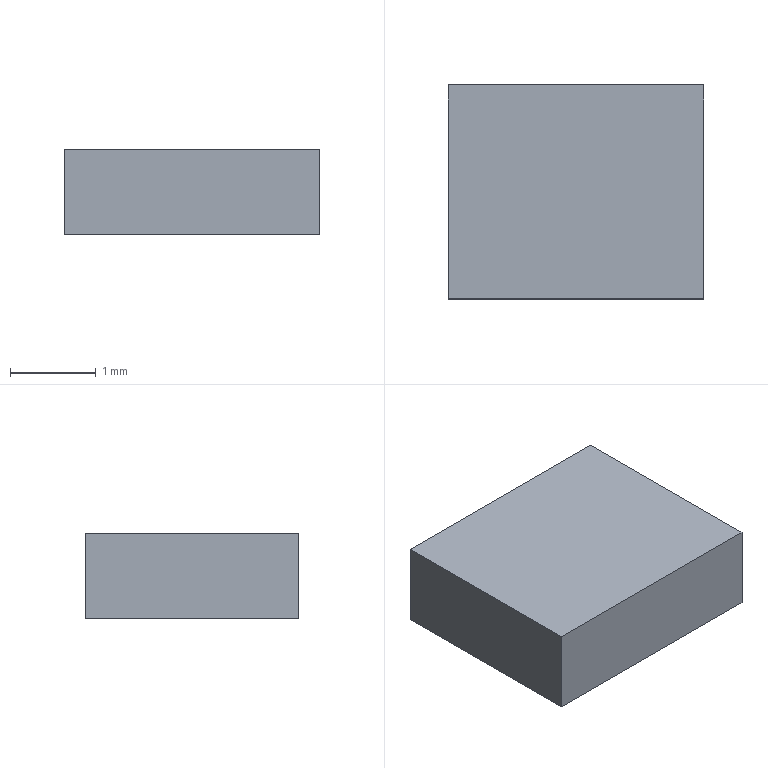Part | Creo | 1 solid | 6 faces | box 2.974 x 2.49 x 1 mm | volume 7.406 mm3 | plane 6
STEP:
#1=CARTESIAN_POINT('',(0.,0.,0.));
#2=DIRECTION('',(0.,0.,1.));
#3=DIRECTION('',(1.,0.,0.));
#4=AXIS2_PLACEMENT_3D('',#1,#2,#3);
#5=CARTESIAN_POINT('',(-1.549,-1.315,0.));
#6=VERTEX_POINT('',#5);
#7=CARTESIAN_POINT('',(1.425,-1.315,0.));
#8=VERTEX_POINT('',#7);
#9=CARTESIAN_POINT('',(-1.549,-1.315,0.));
#10=DIRECTION('',(1.,0.,0.));
#11=VECTOR('',#10,2.974);
#12=LINE('',#9,#11);
#13=EDGE_CURVE('',#6,#8,#12,.T.);
#14=ORIENTED_EDGE('',*,*,#13,.T.);
#15=CARTESIAN_POINT('',(1.425,1.175,0.));
#16=VERTEX_POINT('',#15);
#17=CARTESIAN_POINT('',(1.425,-1.315,0.));
#18=DIRECTION('',(0.,1.,0.));
#19=VECTOR('',#18,2.49);
#20=LINE('',#17,#19);
#21=EDGE_CURVE('',#8,#16,#20,.T.);
#22=ORIENTED_EDGE('',*,*,#21,.T.);
#23=CARTESIAN_POINT('',(-1.549,1.175,0.));
#24=VERTEX_POINT('',#23);
#25=CARTESIAN_POINT('',(1.425,1.175,0.));
#26=DIRECTION('',(-1.,0.,0.));
#27=VECTOR('',#26,2.974);
#28=LINE('',#25,#27);
#29=EDGE_CURVE('',#16,#24,#28,.T.);
#30=ORIENTED_EDGE('',*,*,#29,.T.);
#31=CARTESIAN_POINT('',(-1.549,1.175,0.));
#32=DIRECTION('',(0.,-1.,0.));
#33=VECTOR('',#32,2.49);
#34=LINE('',#31,#33);
#35=EDGE_CURVE('',#24,#6,#34,.T.);
#36=ORIENTED_EDGE('',*,*,#35,.T.);
#37=EDGE_LOOP('',(#14,#22,#30,#36));
#38=FACE_OUTER_BOUND('',#37,.F.);
#39=CARTESIAN_POINT('',(0.,0.,0.));
#40=DIRECTION('',(0.,0.,1.));
#41=DIRECTION('',(1.,0.,0.));
#42=AXIS2_PLACEMENT_3D('',#39,#40,#41);
#43=PLANE('',#42);
#44=ADVANCED_FACE('',(#38),#43,.F.);
#45=ORIENTED_EDGE('',*,*,#13,.F.);
#46=CARTESIAN_POINT('',(-1.549,-1.315,1.));
#47=VERTEX_POINT('',#46);
#48=CARTESIAN_POINT('',(-1.549,-1.315,0.));
#49=DIRECTION('',(0.,0.,1.));
#50=VECTOR('',#49,1.);
#51=LINE('',#48,#50);
#52=EDGE_CURVE('',#6,#47,#51,.T.);
#53=ORIENTED_EDGE('',*,*,#52,.T.);
#54=CARTESIAN_POINT('',(1.425,-1.315,1.));
#55=VERTEX_POINT('',#54);
#56=CARTESIAN_POINT('',(-1.549,-1.315,1.));
#57=DIRECTION('',(1.,0.,0.));
#58=VECTOR('',#57,2.974);
#59=LINE('',#56,#58);
#60=EDGE_CURVE('',#47,#55,#59,.T.);
#61=ORIENTED_EDGE('',*,*,#60,.T.);
#62=CARTESIAN_POINT('',(1.425,-1.315,0.));
#63=DIRECTION('',(0.,0.,1.));
#64=VECTOR('',#63,1.);
#65=LINE('',#62,#64);
#66=EDGE_CURVE('',#8,#55,#65,.T.);
#67=ORIENTED_EDGE('',*,*,#66,.F.);
#68=EDGE_LOOP('',(#45,#53,#61,#67));
#69=FACE_OUTER_BOUND('',#68,.F.);
#70=CARTESIAN_POINT('',(-1.549,-1.315,0.));
#71=DIRECTION('',(0.,-1.,0.));
#72=DIRECTION('',(1.,0.,0.));
#73=AXIS2_PLACEMENT_3D('',#70,#71,#72);
#74=PLANE('',#73);
#75=ADVANCED_FACE('',(#69),#74,.T.);
#76=ORIENTED_EDGE('',*,*,#35,.F.);
#77=CARTESIAN_POINT('',(-1.549,1.175,1.));
#78=VERTEX_POINT('',#77);
#79=CARTESIAN_POINT('',(-1.549,1.175,0.));
#80=DIRECTION('',(0.,0.,1.));
#81=VECTOR('',#80,1.);
#82=LINE('',#79,#81);
#83=EDGE_CURVE('',#24,#78,#82,.T.);
#84=ORIENTED_EDGE('',*,*,#83,.T.);
#85=CARTESIAN_POINT('',(-1.549,1.175,1.));
#86=DIRECTION('',(0.,-1.,0.));
#87=VECTOR('',#86,2.49);
#88=LINE('',#85,#87);
#89=EDGE_CURVE('',#78,#47,#88,.T.);
#90=ORIENTED_EDGE('',*,*,#89,.T.);
#91=ORIENTED_EDGE('',*,*,#52,.F.);
#92=EDGE_LOOP('',(#76,#84,#90,#91));
#93=FACE_OUTER_BOUND('',#92,.F.);
#94=CARTESIAN_POINT('',(-1.549,1.175,0.));
#95=DIRECTION('',(-1.,0.,0.));
#96=DIRECTION('',(0.,-1.,0.));
#97=AXIS2_PLACEMENT_3D('',#94,#95,#96);
#98=PLANE('',#97);
#99=ADVANCED_FACE('',(#93),#98,.T.);
#100=ORIENTED_EDGE('',*,*,#29,.F.);
#101=CARTESIAN_POINT('',(1.425,1.175,1.));
#102=VERTEX_POINT('',#101);
#103=CARTESIAN_POINT('',(1.425,1.175,0.));
#104=DIRECTION('',(0.,0.,1.));
#105=VECTOR('',#104,1.);
#106=LINE('',#103,#105);
#107=EDGE_CURVE('',#16,#102,#106,.T.);
#108=ORIENTED_EDGE('',*,*,#107,.T.);
#109=CARTESIAN_POINT('',(1.425,1.175,1.));
#110=DIRECTION('',(-1.,0.,0.));
#111=VECTOR('',#110,2.974);
#112=LINE('',#109,#111);
#113=EDGE_CURVE('',#102,#78,#112,.T.);
#114=ORIENTED_EDGE('',*,*,#113,.T.);
#115=ORIENTED_EDGE('',*,*,#83,.F.);
#116=EDGE_LOOP('',(#100,#108,#114,#115));
#117=FACE_OUTER_BOUND('',#116,.F.);
#118=CARTESIAN_POINT('',(1.425,1.175,0.));
#119=DIRECTION('',(0.,1.,0.));
#120=DIRECTION('',(-1.,0.,0.));
#121=AXIS2_PLACEMENT_3D('',#118,#119,#120);
#122=PLANE('',#121);
#123=ADVANCED_FACE('',(#117),#122,.T.);
#124=ORIENTED_EDGE('',*,*,#21,.F.);
#125=ORIENTED_EDGE('',*,*,#66,.T.);
#126=CARTESIAN_POINT('',(1.425,-1.315,1.));
#127=DIRECTION('',(0.,1.,0.));
#128=VECTOR('',#127,2.49);
#129=LINE('',#126,#128);
#130=EDGE_CURVE('',#55,#102,#129,.T.);
#131=ORIENTED_EDGE('',*,*,#130,.T.);
#132=ORIENTED_EDGE('',*,*,#107,.F.);
#133=EDGE_LOOP('',(#124,#125,#131,#132));
#134=FACE_OUTER_BOUND('',#133,.F.);
#135=CARTESIAN_POINT('',(1.425,-1.315,0.));
#136=DIRECTION('',(1.,0.,0.));
#137=DIRECTION('',(0.,1.,0.));
#138=AXIS2_PLACEMENT_3D('',#135,#136,#137);
#139=PLANE('',#138);
#140=ADVANCED_FACE('',(#134),#139,.T.);
#141=ORIENTED_EDGE('',*,*,#60,.F.);
#142=ORIENTED_EDGE('',*,*,#89,.F.);
#143=ORIENTED_EDGE('',*,*,#113,.F.);
#144=ORIENTED_EDGE('',*,*,#130,.F.);
#145=EDGE_LOOP('',(#141,#142,#143,#144));
#146=FACE_OUTER_BOUND('',#145,.F.);
#147=CARTESIAN_POINT('',(0.,0.,1.));
#148=DIRECTION('',(0.,0.,1.));
#149=DIRECTION('',(1.,0.,0.));
#150=AXIS2_PLACEMENT_3D('',#147,#148,#149);
#151=PLANE('',#150);
#152=ADVANCED_FACE('',(#146),#151,.T.);
#153=CLOSED_SHELL('',(#44,#75,#99,#123,#140,#152));
#154=MANIFOLD_SOLID_BREP('',#153);
#155=(LENGTH_UNIT()NAMED_UNIT(*)SI_UNIT(.MILLI.,.METRE.));
#156=UNCERTAINTY_MEASURE_WITH_UNIT(LENGTH_MEASURE(0.0004006),#155,'','');
#157=(NAMED_UNIT(*)PLANE_ANGLE_UNIT()SI_UNIT($,.RADIAN.));
#158=PLANE_ANGLE_MEASURE_WITH_UNIT(PLANE_ANGLE_MEASURE(0.01745),#157);
#159=(CONVERSION_BASED_UNIT('DEGREE',#158)NAMED_UNIT(*)PLANE_ANGLE_UNIT());
#160=(NAMED_UNIT(*)SI_UNIT($,.STERADIAN.)SOLID_ANGLE_UNIT());
#161=(GEOMETRIC_REPRESENTATION_CONTEXT(3)GLOBAL_UNCERTAINTY_ASSIGNED_CONTEXT((#156))GLOBAL_UNIT_ASSIGNED_CONTEXT((#155,#159,#160))REPRESENTATION_CONTEXT('',''));
#162=ADVANCED_BREP_SHAPE_REPRESENTATION('',(#4,#154),#161);